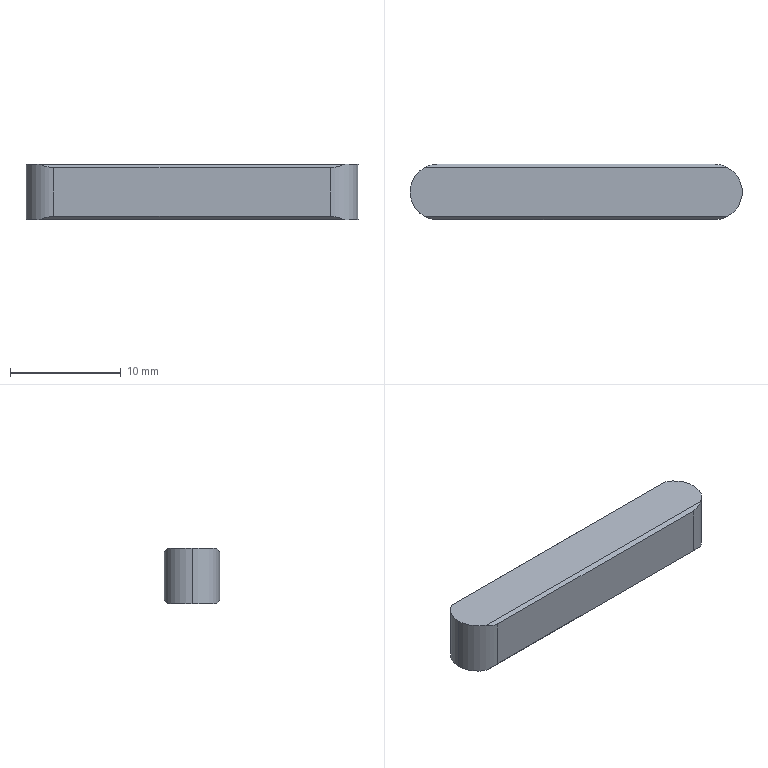Part | STEP file | 0245_004_KESS5-30 | 1 solid | 11 faces | box 30 x 5 x 5 mm | volume 718.443 mm3 | plane 8 | cylinder 3 | commonest cylinder face diameters 5 x3
STEP:
#1=CARTESIAN_POINT('',(0.,0.,0.));
#2=DIRECTION('',(0.,0.,1.));
#3=DIRECTION('',(1.,0.,0.));
#4=AXIS2_PLACEMENT_3D('',#1,#2,#3);
#5=CARTESIAN_POINT('',(0.,2.5,5.));
#6=VERTEX_POINT('',#5);
#7=CARTESIAN_POINT('',(1.313,0.3,5.));
#8=VERTEX_POINT('',#7);
#9=CARTESIAN_POINT('',(2.5,2.5,5.));
#10=DIRECTION('',(0.,0.,1.));
#11=DIRECTION('',(-1.,0.,0.));
#12=AXIS2_PLACEMENT_3D('',#9,#10,#11);
#13=CIRCLE('',#12,2.5);
#14=CARTESIAN_POINT('',(2.5,2.5,0.));
#15=DIRECTION('',(0.,0.,-1.));
#16=DIRECTION('',(-1.,0.,0.));
#17=AXIS2_PLACEMENT_3D('',#14,#15,#16);
#18=CYLINDRICAL_SURFACE('',#17,2.5);
#19=CARTESIAN_POINT('',(6.283,-5.));
#20=DIRECTION('',(-1.,0.));
#21=VECTOR('',#20,1.);
#22=LINE('',#19,#21);
#23=(GEOMETRIC_REPRESENTATION_CONTEXT(2)PARAMETRIC_REPRESENTATION_CONTEXT()REPRESENTATION_CONTEXT('',''));
#24=DEFINITIONAL_REPRESENTATION('',(#22),#23);
#25=PCURVE('',#18,#24);
#26=CARTESIAN_POINT('',(0.,0.,5.));
#27=DIRECTION('',(0.,0.,1.));
#28=DIRECTION('',(1.,0.,0.));
#29=AXIS2_PLACEMENT_3D('',#26,#27,#28);
#30=PLANE('',#29);
#31=CARTESIAN_POINT('',(2.5,2.5));
#32=DIRECTION('',(-1.,0.));
#33=AXIS2_PLACEMENT_2D('',#31,#32);
#34=CIRCLE('',#33,2.5);
#35=(GEOMETRIC_REPRESENTATION_CONTEXT(2)PARAMETRIC_REPRESENTATION_CONTEXT()REPRESENTATION_CONTEXT('',''));
#36=DEFINITIONAL_REPRESENTATION('',(#34),#35);
#37=PCURVE('',#30,#36);
#38=SURFACE_CURVE('',#13,(#25,#37),.PCURVE_S1.);
#39=EDGE_CURVE('',#6,#8,#38,.T.);
#40=ORIENTED_EDGE('',*,*,#39,.F.);
#41=CARTESIAN_POINT('',(0.,2.5,0.));
#42=VERTEX_POINT('',#41);
#43=CARTESIAN_POINT('',(0.,2.5,0.));
#44=DIRECTION('',(0.,0.,-1.));
#45=VECTOR('',#44,1.);
#46=LINE('',#43,#45);
#47=CARTESIAN_POINT('',(6.283,0.));
#48=DIRECTION('',(0.,1.));
#49=VECTOR('',#48,1.);
#50=LINE('',#47,#49);
#51=(GEOMETRIC_REPRESENTATION_CONTEXT(2)PARAMETRIC_REPRESENTATION_CONTEXT()REPRESENTATION_CONTEXT('',''));
#52=DEFINITIONAL_REPRESENTATION('',(#50),#51);
#53=PCURVE('',#18,#52);
#54=CARTESIAN_POINT('',(2.5,2.5,0.));
#55=DIRECTION('',(0.,0.,-1.));
#56=DIRECTION('',(-1.,0.,0.));
#57=AXIS2_PLACEMENT_3D('',#54,#55,#56);
#58=CYLINDRICAL_SURFACE('',#57,2.5);
#59=CARTESIAN_POINT('',(0.,0.));
#60=DIRECTION('',(0.,1.));
#61=VECTOR('',#60,1.);
#62=LINE('',#59,#61);
#63=(GEOMETRIC_REPRESENTATION_CONTEXT(2)PARAMETRIC_REPRESENTATION_CONTEXT()REPRESENTATION_CONTEXT('',''));
#64=DEFINITIONAL_REPRESENTATION('',(#62),#63);
#65=PCURVE('',#58,#64);
#66=SURFACE_CURVE('',#46,(#53,#65),.PCURVE_S1.);
#67=EDGE_CURVE('',#6,#42,#66,.T.);
#68=ORIENTED_EDGE('',*,*,#67,.T.);
#69=CARTESIAN_POINT('',(1.313,0.3,0.));
#70=VERTEX_POINT('',#69);
#71=CARTESIAN_POINT('',(2.5,2.5,0.));
#72=DIRECTION('',(0.,0.,1.));
#73=DIRECTION('',(-1.,0.,0.));
#74=AXIS2_PLACEMENT_3D('',#71,#72,#73);
#75=CIRCLE('',#74,2.5);
#76=CARTESIAN_POINT('',(6.283,0.));
#77=DIRECTION('',(-1.,0.));
#78=VECTOR('',#77,1.);
#79=LINE('',#76,#78);
#80=(GEOMETRIC_REPRESENTATION_CONTEXT(2)PARAMETRIC_REPRESENTATION_CONTEXT()REPRESENTATION_CONTEXT('',''));
#81=DEFINITIONAL_REPRESENTATION('',(#79),#80);
#82=PCURVE('',#18,#81);
#83=CARTESIAN_POINT('',(0.,0.,0.));
#84=DIRECTION('',(0.,0.,1.));
#85=DIRECTION('',(1.,0.,0.));
#86=AXIS2_PLACEMENT_3D('',#83,#84,#85);
#87=PLANE('',#86);
#88=CARTESIAN_POINT('',(2.5,2.5));
#89=DIRECTION('',(-1.,0.));
#90=AXIS2_PLACEMENT_2D('',#88,#89);
#91=CIRCLE('',#90,2.5);
#92=(GEOMETRIC_REPRESENTATION_CONTEXT(2)PARAMETRIC_REPRESENTATION_CONTEXT()REPRESENTATION_CONTEXT('',''));
#93=DEFINITIONAL_REPRESENTATION('',(#91),#92);
#94=PCURVE('',#87,#93);
#95=SURFACE_CURVE('',#75,(#82,#94),.PCURVE_S1.);
#96=EDGE_CURVE('',#42,#70,#95,.T.);
#97=ORIENTED_EDGE('',*,*,#96,.T.);
#98=CARTESIAN_POINT('',(2.5,0.,0.3));
#99=VERTEX_POINT('',#98);
#100=CARTESIAN_POINT('',(1.313,0.3,0.));
#101=CARTESIAN_POINT('',(1.679,0.1021,0.1979));
#102=CARTESIAN_POINT('',(2.083,0.,0.3));
#103=CARTESIAN_POINT('',(2.5,0.,0.3));
#104=(BOUNDED_CURVE()B_SPLINE_CURVE(3,(#100,#101,#102,#103),.UNSPECIFIED.,.F.,.F.)B_SPLINE_CURVE_WITH_KNOTS((4,4),(2.647,3.142),.PIECEWISE_BEZIER_KNOTS.)CURVE()GEOMETRIC_REPRESENTATION_ITEM()RATIONAL_B_SPLINE_CURVE((1.,0.9797,0.9797,1.))REPRESENTATION_ITEM(''));
#105=CARTESIAN_POINT('',(5.207,0.));
#106=CARTESIAN_POINT('',(5.2,-0.008814));
#107=CARTESIAN_POINT('',(5.185,-0.0261));
#108=CARTESIAN_POINT('',(5.163,-0.05099));
#109=CARTESIAN_POINT('',(5.14,-0.07481));
#110=CARTESIAN_POINT('',(5.118,-0.09752));
#111=CARTESIAN_POINT('',(5.095,-0.1191));
#112=CARTESIAN_POINT('',(5.073,-0.1396));
#113=CARTESIAN_POINT('',(5.05,-0.1589));
#114=CARTESIAN_POINT('',(5.028,-0.177));
#115=CARTESIAN_POINT('',(5.005,-0.1939));
#116=CARTESIAN_POINT('',(4.982,-0.2096));
#117=CARTESIAN_POINT('',(4.96,-0.224));
#118=CARTESIAN_POINT('',(4.937,-0.2373));
#119=CARTESIAN_POINT('',(4.915,-0.2493));
#120=CARTESIAN_POINT('',(4.892,-0.26));
#121=CARTESIAN_POINT('',(4.869,-0.2694));
#122=CARTESIAN_POINT('',(4.847,-0.2776));
#123=CARTESIAN_POINT('',(4.824,-0.2845));
#124=CARTESIAN_POINT('',(4.802,-0.2902));
#125=CARTESIAN_POINT('',(4.779,-0.2946));
#126=CARTESIAN_POINT('',(4.757,-0.2977));
#127=CARTESIAN_POINT('',(4.735,-0.2996));
#128=CARTESIAN_POINT('',(4.72,-0.3));
#129=CARTESIAN_POINT('',(4.712,-0.3));
#130=B_SPLINE_CURVE_WITH_KNOTS('',3,(#105,#106,#107,#108,#109,#110,#111,#112,#113,#114,#115,#116,#117,#118,#119,#120,#121,#122,#123,#124,#125,#126,#127,#128,#129),.UNSPECIFIED.,.F.,.F.,(4,1,1,1,1,1,1,1,1,1,1,1,1,1,1,1,1,1,1,1,1,1,4),(2.647,2.669,2.692,2.714,2.737,2.759,2.782,2.804,2.827,2.849,2.872,2.894,2.917,2.939,2.962,2.984,3.007,3.029,3.052,3.074,3.097,3.119,3.142),.QUASI_UNIFORM_KNOTS.);
#131=(GEOMETRIC_REPRESENTATION_CONTEXT(2)PARAMETRIC_REPRESENTATION_CONTEXT()REPRESENTATION_CONTEXT('',''));
#132=DEFINITIONAL_REPRESENTATION('',(#130),#131);
#133=PCURVE('',#18,#132);
#134=CARTESIAN_POINT('',(0.,0.,0.3));
#135=DIRECTION('',(0.,0.7071,0.7071));
#136=DIRECTION('',(0.,-0.7071,0.7071));
#137=AXIS2_PLACEMENT_3D('',#134,#135,#136);
#138=PLANE('',#137);
#139=CARTESIAN_POINT('',(-0.4243,1.313));
#140=CARTESIAN_POINT('',(-0.1444,1.679));
#141=CARTESIAN_POINT('',(0.,2.083));
#142=CARTESIAN_POINT('',(0.,2.5));
#143=(BOUNDED_CURVE()B_SPLINE_CURVE(3,(#139,#140,#141,#142),.UNSPECIFIED.,.F.,.F.)B_SPLINE_CURVE_WITH_KNOTS((4,4),(2.647,3.142),.PIECEWISE_BEZIER_KNOTS.)CURVE()GEOMETRIC_REPRESENTATION_ITEM()RATIONAL_B_SPLINE_CURVE((1.,0.9797,0.9797,1.))REPRESENTATION_ITEM(''));
#144=(GEOMETRIC_REPRESENTATION_CONTEXT(2)PARAMETRIC_REPRESENTATION_CONTEXT()REPRESENTATION_CONTEXT('',''));
#145=DEFINITIONAL_REPRESENTATION('',(#143),#144);
#146=PCURVE('',#138,#145);
#147=SURFACE_CURVE('',#104,(#133,#146),.PCURVE_S1.);
#148=EDGE_CURVE('',#70,#99,#147,.T.);
#149=ORIENTED_EDGE('',*,*,#148,.T.);
#150=CARTESIAN_POINT('',(2.5,0.,4.7));
#151=VERTEX_POINT('',#150);
#152=CARTESIAN_POINT('',(2.5,0.,0.));
#153=DIRECTION('',(0.,0.,1.));
#154=VECTOR('',#153,1.);
#155=LINE('',#152,#154);
#156=CARTESIAN_POINT('',(4.712,0.));
#157=DIRECTION('',(0.,-1.));
#158=VECTOR('',#157,1.);
#159=LINE('',#156,#158);
#160=(GEOMETRIC_REPRESENTATION_CONTEXT(2)PARAMETRIC_REPRESENTATION_CONTEXT()REPRESENTATION_CONTEXT('',''));
#161=DEFINITIONAL_REPRESENTATION('',(#159),#160);
#162=PCURVE('',#18,#161);
#163=CARTESIAN_POINT('',(27.5,0.,0.));
#164=DIRECTION('',(0.,-1.,0.));
#165=DIRECTION('',(0.,0.,-1.));
#166=AXIS2_PLACEMENT_3D('',#163,#164,#165);
#167=PLANE('',#166);
#168=CARTESIAN_POINT('',(0.,-25.));
#169=DIRECTION('',(-1.,0.));
#170=VECTOR('',#169,1.);
#171=LINE('',#168,#170);
#172=(GEOMETRIC_REPRESENTATION_CONTEXT(2)PARAMETRIC_REPRESENTATION_CONTEXT()REPRESENTATION_CONTEXT('',''));
#173=DEFINITIONAL_REPRESENTATION('',(#171),#172);
#174=PCURVE('',#167,#173);
#175=SURFACE_CURVE('',#155,(#162,#174),.PCURVE_S1.);
#176=EDGE_CURVE('',#99,#151,#175,.T.);
#177=ORIENTED_EDGE('',*,*,#176,.T.);
#178=CARTESIAN_POINT('',(2.5,0.,4.7));
#179=CARTESIAN_POINT('',(2.083,0.,4.7));
#180=CARTESIAN_POINT('',(1.679,0.1021,4.802));
#181=CARTESIAN_POINT('',(1.313,0.3,5.));
#182=(BOUNDED_CURVE()B_SPLINE_CURVE(3,(#178,#179,#180,#181),.UNSPECIFIED.,.F.,.F.)B_SPLINE_CURVE_WITH_KNOTS((4,4),(0.,0.4949),.PIECEWISE_BEZIER_KNOTS.)CURVE()GEOMETRIC_REPRESENTATION_ITEM()RATIONAL_B_SPLINE_CURVE((1.,0.9797,0.9797,1.))REPRESENTATION_ITEM(''));
#183=CARTESIAN_POINT('',(4.712,-4.7));
#184=CARTESIAN_POINT('',(4.72,-4.7));
#185=CARTESIAN_POINT('',(4.735,-4.7));
#186=CARTESIAN_POINT('',(4.757,-4.702));
#187=CARTESIAN_POINT('',(4.779,-4.705));
#188=CARTESIAN_POINT('',(4.802,-4.71));
#189=CARTESIAN_POINT('',(4.824,-4.715));
#190=CARTESIAN_POINT('',(4.847,-4.722));
#191=CARTESIAN_POINT('',(4.869,-4.731));
#192=CARTESIAN_POINT('',(4.892,-4.74));
#193=CARTESIAN_POINT('',(4.915,-4.751));
#194=CARTESIAN_POINT('',(4.937,-4.763));
#195=CARTESIAN_POINT('',(4.96,-4.776));
#196=CARTESIAN_POINT('',(4.982,-4.79));
#197=CARTESIAN_POINT('',(5.005,-4.806));
#198=CARTESIAN_POINT('',(5.028,-4.823));
#199=CARTESIAN_POINT('',(5.05,-4.841));
#200=CARTESIAN_POINT('',(5.073,-4.86));
#201=CARTESIAN_POINT('',(5.095,-4.881));
#202=CARTESIAN_POINT('',(5.118,-4.902));
#203=CARTESIAN_POINT('',(5.14,-4.925));
#204=CARTESIAN_POINT('',(5.163,-4.949));
#205=CARTESIAN_POINT('',(5.185,-4.974));
#206=CARTESIAN_POINT('',(5.2,-4.991));
#207=CARTESIAN_POINT('',(5.207,-5.));
#208=B_SPLINE_CURVE_WITH_KNOTS('',3,(#183,#184,#185,#186,#187,#188,#189,#190,#191,#192,#193,#194,#195,#196,#197,#198,#199,#200,#201,#202,#203,#204,#205,#206,#207),.UNSPECIFIED.,.F.,.F.,(4,1,1,1,1,1,1,1,1,1,1,1,1,1,1,1,1,1,1,1,1,1,4),(0.,0.0225,0.04499,0.06749,0.08999,0.1125,0.135,0.1575,0.18,0.2025,0.225,0.2475,0.27,0.2925,0.315,0.3375,0.36,0.3824,0.4049,0.4274,0.4499,0.4724,0.4949),.QUASI_UNIFORM_KNOTS.);
#209=(GEOMETRIC_REPRESENTATION_CONTEXT(2)PARAMETRIC_REPRESENTATION_CONTEXT()REPRESENTATION_CONTEXT('',''));
#210=DEFINITIONAL_REPRESENTATION('',(#208),#209);
#211=PCURVE('',#18,#210);
#212=CARTESIAN_POINT('',(0.,0.3,5.));
#213=DIRECTION('',(0.,0.7071,-0.7071));
#214=DIRECTION('',(0.,0.7071,0.7071));
#215=AXIS2_PLACEMENT_3D('',#212,#213,#214);
#216=PLANE('',#215);
#217=CARTESIAN_POINT('',(-0.4243,2.5));
#218=CARTESIAN_POINT('',(-0.4243,2.083));
#219=CARTESIAN_POINT('',(-0.2799,1.679));
#220=CARTESIAN_POINT('',(0.,1.313));
#221=(BOUNDED_CURVE()B_SPLINE_CURVE(3,(#217,#218,#219,#220),.UNSPECIFIED.,.F.,.F.)B_SPLINE_CURVE_WITH_KNOTS((4,4),(0.,0.4949),.PIECEWISE_BEZIER_KNOTS.)CURVE()GEOMETRIC_REPRESENTATION_ITEM()RATIONAL_B_SPLINE_CURVE((1.,0.9797,0.9797,1.))REPRESENTATION_ITEM(''));
#222=(GEOMETRIC_REPRESENTATION_CONTEXT(2)PARAMETRIC_REPRESENTATION_CONTEXT()REPRESENTATION_CONTEXT('',''));
#223=DEFINITIONAL_REPRESENTATION('',(#221),#222);
#224=PCURVE('',#216,#223);
#225=SURFACE_CURVE('',#182,(#211,#224),.PCURVE_S1.);
#226=EDGE_CURVE('',#151,#8,#225,.T.);
#227=ORIENTED_EDGE('',*,*,#226,.T.);
#228=EDGE_LOOP('',(#40,#68,#97,#149,#177,#227));
#229=FACE_BOUND('',#228,.T.);
#230=ADVANCED_FACE('',(#229),#18,.T.);
#231=CARTESIAN_POINT('',(28.687,4.7,5.));
#232=VERTEX_POINT('',#231);
#233=CARTESIAN_POINT('',(1.313,4.7,5.));
#234=VERTEX_POINT('',#233);
#235=CARTESIAN_POINT('',(0.,4.7,5.));
#236=DIRECTION('',(-1.,0.,0.));
#237=VECTOR('',#236,1.);
#238=LINE('',#235,#237);
#239=CARTESIAN_POINT('',(0.,4.7));
#240=DIRECTION('',(-1.,0.));
#241=VECTOR('',#240,1.);
#242=LINE('',#239,#241);
#243=(GEOMETRIC_REPRESENTATION_CONTEXT(2)PARAMETRIC_REPRESENTATION_CONTEXT()REPRESENTATION_CONTEXT('',''));
#244=DEFINITIONAL_REPRESENTATION('',(#242),#243);
#245=PCURVE('',#30,#244);
#246=CARTESIAN_POINT('',(0.,5.,4.7));
#247=DIRECTION('',(0.,-0.7071,-0.7071));
#248=DIRECTION('',(0.,0.7071,-0.7071));
#249=AXIS2_PLACEMENT_3D('',#246,#247,#248);
#250=PLANE('',#249);
#251=CARTESIAN_POINT('',(-0.4243,0.));
#252=DIRECTION('',(0.,-1.));
#253=VECTOR('',#252,1.);
#254=LINE('',#251,#253);
#255=(GEOMETRIC_REPRESENTATION_CONTEXT(2)PARAMETRIC_REPRESENTATION_CONTEXT()REPRESENTATION_CONTEXT('',''));
#256=DEFINITIONAL_REPRESENTATION('',(#254),#255);
#257=PCURVE('',#250,#256);
#258=SURFACE_CURVE('',#238,(#245,#257),.PCURVE_S1.);
#259=EDGE_CURVE('',#232,#234,#258,.T.);
#260=ORIENTED_EDGE('',*,*,#259,.T.);
#261=CARTESIAN_POINT('',(2.5,2.5,5.));
#262=DIRECTION('',(0.,0.,1.));
#263=DIRECTION('',(-1.,0.,0.));
#264=AXIS2_PLACEMENT_3D('',#261,#262,#263);
#265=CIRCLE('',#264,2.5);
#266=CARTESIAN_POINT('',(2.5,2.5));
#267=DIRECTION('',(-1.,0.));
#268=AXIS2_PLACEMENT_2D('',#266,#267);
#269=CIRCLE('',#268,2.5);
#270=(GEOMETRIC_REPRESENTATION_CONTEXT(2)PARAMETRIC_REPRESENTATION_CONTEXT()REPRESENTATION_CONTEXT('',''));
#271=DEFINITIONAL_REPRESENTATION('',(#269),#270);
#272=PCURVE('',#30,#271);
#273=CARTESIAN_POINT('',(6.283,-5.));
#274=DIRECTION('',(-1.,0.));
#275=VECTOR('',#274,1.);
#276=LINE('',#273,#275);
#277=(GEOMETRIC_REPRESENTATION_CONTEXT(2)PARAMETRIC_REPRESENTATION_CONTEXT()REPRESENTATION_CONTEXT('',''));
#278=DEFINITIONAL_REPRESENTATION('',(#276),#277);
#279=PCURVE('',#58,#278);
#280=SURFACE_CURVE('',#265,(#272,#279),.PCURVE_S1.);
#281=EDGE_CURVE('',#234,#6,#280,.T.);
#282=ORIENTED_EDGE('',*,*,#281,.T.);
#283=ORIENTED_EDGE('',*,*,#39,.T.);
#284=CARTESIAN_POINT('',(28.687,0.3,5.));
#285=VERTEX_POINT('',#284);
#286=CARTESIAN_POINT('',(0.,0.3,5.));
#287=DIRECTION('',(1.,0.,0.));
#288=VECTOR('',#287,1.);
#289=LINE('',#286,#288);
#290=CARTESIAN_POINT('',(0.,0.3));
#291=DIRECTION('',(1.,0.));
#292=VECTOR('',#291,1.);
#293=LINE('',#290,#292);
#294=(GEOMETRIC_REPRESENTATION_CONTEXT(2)PARAMETRIC_REPRESENTATION_CONTEXT()REPRESENTATION_CONTEXT('',''));
#295=DEFINITIONAL_REPRESENTATION('',(#293),#294);
#296=PCURVE('',#30,#295);
#297=CARTESIAN_POINT('',(0.,0.));
#298=DIRECTION('',(0.,1.));
#299=VECTOR('',#298,1.);
#300=LINE('',#297,#299);
#301=(GEOMETRIC_REPRESENTATION_CONTEXT(2)PARAMETRIC_REPRESENTATION_CONTEXT()REPRESENTATION_CONTEXT('',''));
#302=DEFINITIONAL_REPRESENTATION('',(#300),#301);
#303=PCURVE('',#216,#302);
#304=SURFACE_CURVE('',#289,(#296,#303),.PCURVE_S1.);
#305=EDGE_CURVE('',#8,#285,#304,.T.);
#306=ORIENTED_EDGE('',*,*,#305,.T.);
#307=CARTESIAN_POINT('',(27.5,2.5,5.));
#308=DIRECTION('',(0.,0.,1.));
#309=DIRECTION('',(-1.,0.,0.));
#310=AXIS2_PLACEMENT_3D('',#307,#308,#309);
#311=CIRCLE('',#310,2.5);
#312=CARTESIAN_POINT('',(27.5,2.5));
#313=DIRECTION('',(-1.,0.));
#314=AXIS2_PLACEMENT_2D('',#312,#313);
#315=CIRCLE('',#314,2.5);
#316=(GEOMETRIC_REPRESENTATION_CONTEXT(2)PARAMETRIC_REPRESENTATION_CONTEXT()REPRESENTATION_CONTEXT('',''));
#317=DEFINITIONAL_REPRESENTATION('',(#315),#316);
#318=PCURVE('',#30,#317);
#319=CARTESIAN_POINT('',(27.5,2.5,0.));
#320=DIRECTION('',(0.,0.,-1.));
#321=DIRECTION('',(-1.,0.,0.));
#322=AXIS2_PLACEMENT_3D('',#319,#320,#321);
#323=CYLINDRICAL_SURFACE('',#322,2.5);
#324=CARTESIAN_POINT('',(6.283,-5.));
#325=DIRECTION('',(-1.,0.));
#326=VECTOR('',#325,1.);
#327=LINE('',#324,#326);
#328=(GEOMETRIC_REPRESENTATION_CONTEXT(2)PARAMETRIC_REPRESENTATION_CONTEXT()REPRESENTATION_CONTEXT('',''));
#329=DEFINITIONAL_REPRESENTATION('',(#327),#328);
#330=PCURVE('',#323,#329);
#331=SURFACE_CURVE('',#311,(#318,#330),.PCURVE_S1.);
#332=EDGE_CURVE('',#285,#232,#331,.T.);
#333=ORIENTED_EDGE('',*,*,#332,.T.);
#334=EDGE_LOOP('',(#260,#282,#283,#306,#333));
#335=FACE_BOUND('',#334,.T.);
#336=ADVANCED_FACE('',(#335),#30,.T.);
#337=ORIENTED_EDGE('',*,*,#67,.F.);
#338=ORIENTED_EDGE('',*,*,#281,.F.);
#339=CARTESIAN_POINT('',(2.5,5.,4.7));
#340=VERTEX_POINT('',#339);
#341=CARTESIAN_POINT('',(1.313,4.7,5.));
#342=CARTESIAN_POINT('',(1.679,4.898,4.802));
#343=CARTESIAN_POINT('',(2.083,5.,4.7));
#344=CARTESIAN_POINT('',(2.5,5.,4.7));
#345=(BOUNDED_CURVE()B_SPLINE_CURVE(3,(#341,#342,#343,#344),.UNSPECIFIED.,.F.,.F.)B_SPLINE_CURVE_WITH_KNOTS((4,4),(5.788,6.283),.PIECEWISE_BEZIER_KNOTS.)CURVE()GEOMETRIC_REPRESENTATION_ITEM()RATIONAL_B_SPLINE_CURVE((1.,0.9797,0.9797,1.))REPRESENTATION_ITEM(''));
#346=CARTESIAN_POINT('',(1.076,-5.));
#347=CARTESIAN_POINT('',(1.083,-4.991));
#348=CARTESIAN_POINT('',(1.098,-4.974));
#349=CARTESIAN_POINT('',(1.121,-4.949));
#350=CARTESIAN_POINT('',(1.143,-4.925));
#351=CARTESIAN_POINT('',(1.165,-4.902));
#352=CARTESIAN_POINT('',(1.188,-4.881));
#353=CARTESIAN_POINT('',(1.21,-4.86));
#354=CARTESIAN_POINT('',(1.233,-4.841));
#355=CARTESIAN_POINT('',(1.256,-4.823));
#356=CARTESIAN_POINT('',(1.278,-4.806));
#357=CARTESIAN_POINT('',(1.301,-4.79));
#358=CARTESIAN_POINT('',(1.323,-4.776));
#359=CARTESIAN_POINT('',(1.346,-4.763));
#360=CARTESIAN_POINT('',(1.369,-4.751));
#361=CARTESIAN_POINT('',(1.391,-4.74));
#362=CARTESIAN_POINT('',(1.414,-4.731));
#363=CARTESIAN_POINT('',(1.436,-4.722));
#364=CARTESIAN_POINT('',(1.459,-4.715));
#365=CARTESIAN_POINT('',(1.481,-4.71));
#366=CARTESIAN_POINT('',(1.504,-4.705));
#367=CARTESIAN_POINT('',(1.526,-4.702));
#368=CARTESIAN_POINT('',(1.549,-4.7));
#369=CARTESIAN_POINT('',(1.563,-4.7));
#370=CARTESIAN_POINT('',(1.571,-4.7));
#371=B_SPLINE_CURVE_WITH_KNOTS('',3,(#346,#347,#348,#349,#350,#351,#352,#353,#354,#355,#356,#357,#358,#359,#360,#361,#362,#363,#364,#365,#366,#367,#368,#369,#370),.UNSPECIFIED.,.F.,.F.,(4,1,1,1,1,1,1,1,1,1,1,1,1,1,1,1,1,1,1,1,1,1,4),(5.788,5.811,5.833,5.856,5.878,5.901,5.923,5.946,5.968,5.991,6.013,6.036,6.058,6.081,6.103,6.126,6.148,6.171,6.193,6.216,6.238,6.261,6.283),.QUASI_UNIFORM_KNOTS.);
#372=(GEOMETRIC_REPRESENTATION_CONTEXT(2)PARAMETRIC_REPRESENTATION_CONTEXT()REPRESENTATION_CONTEXT('',''));
#373=DEFINITIONAL_REPRESENTATION('',(#371),#372);
#374=PCURVE('',#58,#373);
#375=CARTESIAN_POINT('',(-0.4243,1.313));
#376=CARTESIAN_POINT('',(-0.1444,1.679));
#377=CARTESIAN_POINT('',(0.,2.083));
#378=CARTESIAN_POINT('',(0.,2.5));
#379=(BOUNDED_CURVE()B_SPLINE_CURVE(3,(#375,#376,#377,#378),.UNSPECIFIED.,.F.,.F.)B_SPLINE_CURVE_WITH_KNOTS((4,4),(5.788,6.283),.PIECEWISE_BEZIER_KNOTS.)CURVE()GEOMETRIC_REPRESENTATION_ITEM()RATIONAL_B_SPLINE_CURVE((1.,0.9797,0.9797,1.))REPRESENTATION_ITEM(''));
#380=(GEOMETRIC_REPRESENTATION_CONTEXT(2)PARAMETRIC_REPRESENTATION_CONTEXT()REPRESENTATION_CONTEXT('',''));
#381=DEFINITIONAL_REPRESENTATION('',(#379),#380);
#382=PCURVE('',#250,#381);
#383=SURFACE_CURVE('',#345,(#374,#382),.PCURVE_S1.);
#384=EDGE_CURVE('',#234,#340,#383,.T.);
#385=ORIENTED_EDGE('',*,*,#384,.T.);
#386=CARTESIAN_POINT('',(2.5,5.,0.3));
#387=VERTEX_POINT('',#386);
#388=CARTESIAN_POINT('',(2.5,5.,0.));
#389=DIRECTION('',(0.,0.,-1.));
#390=VECTOR('',#389,1.);
#391=LINE('',#388,#390);
#392=CARTESIAN_POINT('',(1.571,0.));
#393=DIRECTION('',(0.,1.));
#394=VECTOR('',#393,1.);
#395=LINE('',#392,#394);
#396=(GEOMETRIC_REPRESENTATION_CONTEXT(2)PARAMETRIC_REPRESENTATION_CONTEXT()REPRESENTATION_CONTEXT('',''));
#397=DEFINITIONAL_REPRESENTATION('',(#395),#396);
#398=PCURVE('',#58,#397);
#399=CARTESIAN_POINT('',(2.5,5.,0.));
#400=DIRECTION('',(0.,1.,0.));
#401=DIRECTION('',(0.,0.,1.));
#402=AXIS2_PLACEMENT_3D('',#399,#400,#401);
#403=PLANE('',#402);
#404=CARTESIAN_POINT('',(0.,0.));
#405=DIRECTION('',(-1.,0.));
#406=VECTOR('',#405,1.);
#407=LINE('',#404,#406);
#408=(GEOMETRIC_REPRESENTATION_CONTEXT(2)PARAMETRIC_REPRESENTATION_CONTEXT()REPRESENTATION_CONTEXT('',''));
#409=DEFINITIONAL_REPRESENTATION('',(#407),#408);
#410=PCURVE('',#403,#409);
#411=SURFACE_CURVE('',#391,(#398,#410),.PCURVE_S1.);
#412=EDGE_CURVE('',#340,#387,#411,.T.);
#413=ORIENTED_EDGE('',*,*,#412,.T.);
#414=CARTESIAN_POINT('',(1.313,4.7,0.));
#415=VERTEX_POINT('',#414);
#416=CARTESIAN_POINT('',(2.5,5.,0.3));
#417=CARTESIAN_POINT('',(2.083,5.,0.3));
#418=CARTESIAN_POINT('',(1.679,4.898,0.1979));
#419=CARTESIAN_POINT('',(1.313,4.7,0.));
#420=(BOUNDED_CURVE()B_SPLINE_CURVE(3,(#416,#417,#418,#419),.UNSPECIFIED.,.F.,.F.)B_SPLINE_CURVE_WITH_KNOTS((4,4),(3.142,3.637),.PIECEWISE_BEZIER_KNOTS.)CURVE()GEOMETRIC_REPRESENTATION_ITEM()RATIONAL_B_SPLINE_CURVE((1.,0.9797,0.9797,1.))REPRESENTATION_ITEM(''));
#421=CARTESIAN_POINT('',(1.571,-0.3));
#422=CARTESIAN_POINT('',(1.563,-0.3));
#423=CARTESIAN_POINT('',(1.549,-0.2996));
#424=CARTESIAN_POINT('',(1.526,-0.2977));
#425=CARTESIAN_POINT('',(1.504,-0.2946));
#426=CARTESIAN_POINT('',(1.481,-0.2902));
#427=CARTESIAN_POINT('',(1.459,-0.2845));
#428=CARTESIAN_POINT('',(1.436,-0.2776));
#429=CARTESIAN_POINT('',(1.414,-0.2694));
#430=CARTESIAN_POINT('',(1.391,-0.26));
#431=CARTESIAN_POINT('',(1.369,-0.2493));
#432=CARTESIAN_POINT('',(1.346,-0.2373));
#433=CARTESIAN_POINT('',(1.323,-0.224));
#434=CARTESIAN_POINT('',(1.301,-0.2096));
#435=CARTESIAN_POINT('',(1.278,-0.1939));
#436=CARTESIAN_POINT('',(1.256,-0.177));
#437=CARTESIAN_POINT('',(1.233,-0.1589));
#438=CARTESIAN_POINT('',(1.21,-0.1396));
#439=CARTESIAN_POINT('',(1.188,-0.1191));
#440=CARTESIAN_POINT('',(1.165,-0.09752));
#441=CARTESIAN_POINT('',(1.143,-0.07481));
#442=CARTESIAN_POINT('',(1.121,-0.05099));
#443=CARTESIAN_POINT('',(1.098,-0.0261));
#444=CARTESIAN_POINT('',(1.083,-0.008814));
#445=CARTESIAN_POINT('',(1.076,0.));
#446=B_SPLINE_CURVE_WITH_KNOTS('',3,(#421,#422,#423,#424,#425,#426,#427,#428,#429,#430,#431,#432,#433,#434,#435,#436,#437,#438,#439,#440,#441,#442,#443,#444,#445),.UNSPECIFIED.,.F.,.F.,(4,1,1,1,1,1,1,1,1,1,1,1,1,1,1,1,1,1,1,1,1,1,4),(3.142,3.164,3.187,3.209,3.232,3.254,3.277,3.299,3.322,3.344,3.367,3.389,3.412,3.434,3.457,3.479,3.502,3.524,3.547,3.569,3.592,3.614,3.637),.QUASI_UNIFORM_KNOTS.);
#447=(GEOMETRIC_REPRESENTATION_CONTEXT(2)PARAMETRIC_REPRESENTATION_CONTEXT()REPRESENTATION_CONTEXT('',''));
#448=DEFINITIONAL_REPRESENTATION('',(#446),#447);
#449=PCURVE('',#58,#448);
#450=CARTESIAN_POINT('',(0.,4.7,0.));
#451=DIRECTION('',(0.,-0.7071,0.7071));
#452=DIRECTION('',(0.,-0.7071,-0.7071));
#453=AXIS2_PLACEMENT_3D('',#450,#451,#452);
#454=PLANE('',#453);
#455=CARTESIAN_POINT('',(-0.4243,2.5));
#456=CARTESIAN_POINT('',(-0.4243,2.083));
#457=CARTESIAN_POINT('',(-0.2799,1.679));
#458=CARTESIAN_POINT('',(0.,1.313));
#459=(BOUNDED_CURVE()B_SPLINE_CURVE(3,(#455,#456,#457,#458),.UNSPECIFIED.,.F.,.F.)B_SPLINE_CURVE_WITH_KNOTS((4,4),(3.142,3.637),.PIECEWISE_BEZIER_KNOTS.)CURVE()GEOMETRIC_REPRESENTATION_ITEM()RATIONAL_B_SPLINE_CURVE((1.,0.9797,0.9797,1.))REPRESENTATION_ITEM(''));
#460=(GEOMETRIC_REPRESENTATION_CONTEXT(2)PARAMETRIC_REPRESENTATION_CONTEXT()REPRESENTATION_CONTEXT('',''));
#461=DEFINITIONAL_REPRESENTATION('',(#459),#460);
#462=PCURVE('',#454,#461);
#463=SURFACE_CURVE('',#420,(#449,#462),.PCURVE_S1.);
#464=EDGE_CURVE('',#387,#415,#463,.T.);
#465=ORIENTED_EDGE('',*,*,#464,.T.);
#466=CARTESIAN_POINT('',(2.5,2.5,0.));
#467=DIRECTION('',(0.,0.,1.));
#468=DIRECTION('',(-1.,0.,0.));
#469=AXIS2_PLACEMENT_3D('',#466,#467,#468);
#470=CIRCLE('',#469,2.5);
#471=CARTESIAN_POINT('',(6.283,0.));
#472=DIRECTION('',(-1.,0.));
#473=VECTOR('',#472,1.);
#474=LINE('',#471,#473);
#475=(GEOMETRIC_REPRESENTATION_CONTEXT(2)PARAMETRIC_REPRESENTATION_CONTEXT()REPRESENTATION_CONTEXT('',''));
#476=DEFINITIONAL_REPRESENTATION('',(#474),#475);
#477=PCURVE('',#58,#476);
#478=CARTESIAN_POINT('',(2.5,2.5));
#479=DIRECTION('',(-1.,0.));
#480=AXIS2_PLACEMENT_2D('',#478,#479);
#481=CIRCLE('',#480,2.5);
#482=(GEOMETRIC_REPRESENTATION_CONTEXT(2)PARAMETRIC_REPRESENTATION_CONTEXT()REPRESENTATION_CONTEXT('',''));
#483=DEFINITIONAL_REPRESENTATION('',(#481),#482);
#484=PCURVE('',#87,#483);
#485=SURFACE_CURVE('',#470,(#477,#484),.PCURVE_S1.);
#486=EDGE_CURVE('',#415,#42,#485,.T.);
#487=ORIENTED_EDGE('',*,*,#486,.T.);
#488=EDGE_LOOP('',(#337,#338,#385,#413,#465,#487));
#489=FACE_BOUND('',#488,.T.);
#490=ADVANCED_FACE('',(#489),#58,.T.);
#491=CARTESIAN_POINT('',(27.5,5.,4.7));
#492=VERTEX_POINT('',#491);
#493=CARTESIAN_POINT('',(0.,5.,4.7));
#494=DIRECTION('',(1.,0.,0.));
#495=VECTOR('',#494,1.);
#496=LINE('',#493,#495);
#497=CARTESIAN_POINT('',(0.,0.));
#498=DIRECTION('',(0.,1.));
#499=VECTOR('',#498,1.);
#500=LINE('',#497,#499);
#501=(GEOMETRIC_REPRESENTATION_CONTEXT(2)PARAMETRIC_REPRESENTATION_CONTEXT()REPRESENTATION_CONTEXT('',''));
#502=DEFINITIONAL_REPRESENTATION('',(#500),#501);
#503=PCURVE('',#250,#502);
#504=CARTESIAN_POINT('',(4.7,-2.5));
#505=DIRECTION('',(0.,1.));
#506=VECTOR('',#505,1.);
#507=LINE('',#504,#506);
#508=(GEOMETRIC_REPRESENTATION_CONTEXT(2)PARAMETRIC_REPRESENTATION_CONTEXT()REPRESENTATION_CONTEXT('',''));
#509=DEFINITIONAL_REPRESENTATION('',(#507),#508);
#510=PCURVE('',#403,#509);
#511=SURFACE_CURVE('',#496,(#503,#510),.PCURVE_S1.);
#512=EDGE_CURVE('',#340,#492,#511,.T.);
#513=ORIENTED_EDGE('',*,*,#512,.F.);
#514=ORIENTED_EDGE('',*,*,#384,.F.);
#515=ORIENTED_EDGE('',*,*,#259,.F.);
#516=CARTESIAN_POINT('',(27.5,5.,4.7));
#517=CARTESIAN_POINT('',(27.917,5.,4.7));
#518=CARTESIAN_POINT('',(28.321,4.898,4.802));
#519=CARTESIAN_POINT('',(28.687,4.7,5.));
#520=(BOUNDED_CURVE()B_SPLINE_CURVE(3,(#516,#517,#518,#519),.UNSPECIFIED.,.F.,.F.)B_SPLINE_CURVE_WITH_KNOTS((4,4),(0.,0.4949),.PIECEWISE_BEZIER_KNOTS.)CURVE()GEOMETRIC_REPRESENTATION_ITEM()RATIONAL_B_SPLINE_CURVE((1.,0.9797,0.9797,1.))REPRESENTATION_ITEM(''));
#521=CARTESIAN_POINT('',(0.,27.5));
#522=CARTESIAN_POINT('',(0.,27.917));
#523=CARTESIAN_POINT('',(-0.1444,28.321));
#524=CARTESIAN_POINT('',(-0.4243,28.687));
#525=(BOUNDED_CURVE()B_SPLINE_CURVE(3,(#521,#522,#523,#524),.UNSPECIFIED.,.F.,.F.)B_SPLINE_CURVE_WITH_KNOTS((4,4),(0.,0.4949),.PIECEWISE_BEZIER_KNOTS.)CURVE()GEOMETRIC_REPRESENTATION_ITEM()RATIONAL_B_SPLINE_CURVE((1.,0.9797,0.9797,1.))REPRESENTATION_ITEM(''));
#526=(GEOMETRIC_REPRESENTATION_CONTEXT(2)PARAMETRIC_REPRESENTATION_CONTEXT()REPRESENTATION_CONTEXT('',''));
#527=DEFINITIONAL_REPRESENTATION('',(#525),#526);
#528=PCURVE('',#250,#527);
#529=CARTESIAN_POINT('',(1.571,-4.7));
#530=CARTESIAN_POINT('',(1.578,-4.7));
#531=CARTESIAN_POINT('',(1.593,-4.7));
#532=CARTESIAN_POINT('',(1.615,-4.702));
#533=CARTESIAN_POINT('',(1.638,-4.705));
#534=CARTESIAN_POINT('',(1.66,-4.71));
#535=CARTESIAN_POINT('',(1.683,-4.715));
#536=CARTESIAN_POINT('',(1.705,-4.722));
#537=CARTESIAN_POINT('',(1.728,-4.731));
#538=CARTESIAN_POINT('',(1.75,-4.74));
#539=CARTESIAN_POINT('',(1.773,-4.751));
#540=CARTESIAN_POINT('',(1.796,-4.763));
#541=CARTESIAN_POINT('',(1.818,-4.776));
#542=CARTESIAN_POINT('',(1.841,-4.79));
#543=CARTESIAN_POINT('',(1.863,-4.806));
#544=CARTESIAN_POINT('',(1.886,-4.823));
#545=CARTESIAN_POINT('',(1.909,-4.841));
#546=CARTESIAN_POINT('',(1.931,-4.86));
#547=CARTESIAN_POINT('',(1.954,-4.881));
#548=CARTESIAN_POINT('',(1.976,-4.902));
#549=CARTESIAN_POINT('',(1.999,-4.925));
#550=CARTESIAN_POINT('',(2.021,-4.949));
#551=CARTESIAN_POINT('',(2.043,-4.974));
#552=CARTESIAN_POINT('',(2.058,-4.991));
#553=CARTESIAN_POINT('',(2.066,-5.));
#554=B_SPLINE_CURVE_WITH_KNOTS('',3,(#529,#530,#531,#532,#533,#534,#535,#536,#537,#538,#539,#540,#541,#542,#543,#544,#545,#546,#547,#548,#549,#550,#551,#552,#553),.UNSPECIFIED.,.F.,.F.,(4,1,1,1,1,1,1,1,1,1,1,1,1,1,1,1,1,1,1,1,1,1,4),(0.,0.0225,0.04499,0.06749,0.08999,0.1125,0.135,0.1575,0.18,0.2025,0.225,0.2475,0.27,0.2925,0.315,0.3375,0.36,0.3824,0.4049,0.4274,0.4499,0.4724,0.4949),.QUASI_UNIFORM_KNOTS.);
#555=(GEOMETRIC_REPRESENTATION_CONTEXT(2)PARAMETRIC_REPRESENTATION_CONTEXT()REPRESENTATION_CONTEXT('',''));
#556=DEFINITIONAL_REPRESENTATION('',(#554),#555);
#557=PCURVE('',#323,#556);
#558=SURFACE_CURVE('',#520,(#528,#557),.PCURVE_S1.);
#559=EDGE_CURVE('',#492,#232,#558,.T.);
#560=ORIENTED_EDGE('',*,*,#559,.F.);
#561=EDGE_LOOP('',(#513,#514,#515,#560));
#562=FACE_BOUND('',#561,.T.);
#563=ADVANCED_FACE('',(#562),#250,.F.);
#564=ORIENTED_EDGE('',*,*,#559,.T.);
#565=ORIENTED_EDGE('',*,*,#332,.F.);
#566=CARTESIAN_POINT('',(27.5,0.,4.7));
#567=VERTEX_POINT('',#566);
#568=CARTESIAN_POINT('',(28.687,0.3,5.));
#569=CARTESIAN_POINT('',(28.321,0.1021,4.802));
#570=CARTESIAN_POINT('',(27.917,0.,4.7));
#571=CARTESIAN_POINT('',(27.5,0.,4.7));
#572=(BOUNDED_CURVE()B_SPLINE_CURVE(3,(#568,#569,#570,#571),.UNSPECIFIED.,.F.,.F.)B_SPLINE_CURVE_WITH_KNOTS((4,4),(5.788,6.283),.PIECEWISE_BEZIER_KNOTS.)CURVE()GEOMETRIC_REPRESENTATION_ITEM()RATIONAL_B_SPLINE_CURVE((1.,0.9797,0.9797,1.))REPRESENTATION_ITEM(''));
#573=CARTESIAN_POINT('',(4.217,-5.));
#574=CARTESIAN_POINT('',(4.225,-4.991));
#575=CARTESIAN_POINT('',(4.24,-4.974));
#576=CARTESIAN_POINT('',(4.262,-4.949));
#577=CARTESIAN_POINT('',(4.285,-4.925));
#578=CARTESIAN_POINT('',(4.307,-4.902));
#579=CARTESIAN_POINT('',(4.329,-4.881));
#580=CARTESIAN_POINT('',(4.352,-4.86));
#581=CARTESIAN_POINT('',(4.375,-4.841));
#582=CARTESIAN_POINT('',(4.397,-4.823));
#583=CARTESIAN_POINT('',(4.42,-4.806));
#584=CARTESIAN_POINT('',(4.442,-4.79));
#585=CARTESIAN_POINT('',(4.465,-4.776));
#586=CARTESIAN_POINT('',(4.488,-4.763));
#587=CARTESIAN_POINT('',(4.51,-4.751));
#588=CARTESIAN_POINT('',(4.533,-4.74));
#589=CARTESIAN_POINT('',(4.555,-4.731));
#590=CARTESIAN_POINT('',(4.578,-4.722));
#591=CARTESIAN_POINT('',(4.6,-4.715));
#592=CARTESIAN_POINT('',(4.623,-4.71));
#593=CARTESIAN_POINT('',(4.645,-4.705));
#594=CARTESIAN_POINT('',(4.668,-4.702));
#595=CARTESIAN_POINT('',(4.69,-4.7));
#596=CARTESIAN_POINT('',(4.705,-4.7));
#597=CARTESIAN_POINT('',(4.712,-4.7));
#598=B_SPLINE_CURVE_WITH_KNOTS('',3,(#573,#574,#575,#576,#577,#578,#579,#580,#581,#582,#583,#584,#585,#586,#587,#588,#589,#590,#591,#592,#593,#594,#595,#596,#597),.UNSPECIFIED.,.F.,.F.,(4,1,1,1,1,1,1,1,1,1,1,1,1,1,1,1,1,1,1,1,1,1,4),(5.788,5.811,5.833,5.856,5.878,5.901,5.923,5.946,5.968,5.991,6.013,6.036,6.058,6.081,6.103,6.126,6.148,6.171,6.193,6.216,6.238,6.261,6.283),.QUASI_UNIFORM_KNOTS.);
#599=(GEOMETRIC_REPRESENTATION_CONTEXT(2)PARAMETRIC_REPRESENTATION_CONTEXT()REPRESENTATION_CONTEXT('',''));
#600=DEFINITIONAL_REPRESENTATION('',(#598),#599);
#601=PCURVE('',#323,#600);
#602=CARTESIAN_POINT('',(0.,28.687));
#603=CARTESIAN_POINT('',(-0.2799,28.321));
#604=CARTESIAN_POINT('',(-0.4243,27.917));
#605=CARTESIAN_POINT('',(-0.4243,27.5));
#606=(BOUNDED_CURVE()B_SPLINE_CURVE(3,(#602,#603,#604,#605),.UNSPECIFIED.,.F.,.F.)B_SPLINE_CURVE_WITH_KNOTS((4,4),(5.788,6.283),.PIECEWISE_BEZIER_KNOTS.)CURVE()GEOMETRIC_REPRESENTATION_ITEM()RATIONAL_B_SPLINE_CURVE((1.,0.9797,0.9797,1.))REPRESENTATION_ITEM(''));
#607=(GEOMETRIC_REPRESENTATION_CONTEXT(2)PARAMETRIC_REPRESENTATION_CONTEXT()REPRESENTATION_CONTEXT('',''));
#608=DEFINITIONAL_REPRESENTATION('',(#606),#607);
#609=PCURVE('',#216,#608);
#610=SURFACE_CURVE('',#572,(#601,#609),.PCURVE_S1.);
#611=EDGE_CURVE('',#285,#567,#610,.T.);
#612=ORIENTED_EDGE('',*,*,#611,.T.);
#613=CARTESIAN_POINT('',(27.5,0.,0.3));
#614=VERTEX_POINT('',#613);
#615=CARTESIAN_POINT('',(27.5,0.,0.));
#616=DIRECTION('',(0.,0.,-1.));
#617=VECTOR('',#616,1.);
#618=LINE('',#615,#617);
#619=CARTESIAN_POINT('',(4.712,0.));
#620=DIRECTION('',(0.,1.));
#621=VECTOR('',#620,1.);
#622=LINE('',#619,#621);
#623=(GEOMETRIC_REPRESENTATION_CONTEXT(2)PARAMETRIC_REPRESENTATION_CONTEXT()REPRESENTATION_CONTEXT('',''));
#624=DEFINITIONAL_REPRESENTATION('',(#622),#623);
#625=PCURVE('',#323,#624);
#626=CARTESIAN_POINT('',(0.,0.));
#627=DIRECTION('',(1.,0.));
#628=VECTOR('',#627,1.);
#629=LINE('',#626,#628);
#630=(GEOMETRIC_REPRESENTATION_CONTEXT(2)PARAMETRIC_REPRESENTATION_CONTEXT()REPRESENTATION_CONTEXT('',''));
#631=DEFINITIONAL_REPRESENTATION('',(#629),#630);
#632=PCURVE('',#167,#631);
#633=SURFACE_CURVE('',#618,(#625,#632),.PCURVE_S1.);
#634=EDGE_CURVE('',#567,#614,#633,.T.);
#635=ORIENTED_EDGE('',*,*,#634,.T.);
#636=CARTESIAN_POINT('',(28.687,0.3,0.));
#637=VERTEX_POINT('',#636);
#638=CARTESIAN_POINT('',(27.5,0.,0.3));
#639=CARTESIAN_POINT('',(27.917,0.,0.3));
#640=CARTESIAN_POINT('',(28.321,0.1021,0.1979));
#641=CARTESIAN_POINT('',(28.687,0.3,0.));
#642=(BOUNDED_CURVE()B_SPLINE_CURVE(3,(#638,#639,#640,#641),.UNSPECIFIED.,.F.,.F.)B_SPLINE_CURVE_WITH_KNOTS((4,4),(3.142,3.637),.PIECEWISE_BEZIER_KNOTS.)CURVE()GEOMETRIC_REPRESENTATION_ITEM()RATIONAL_B_SPLINE_CURVE((1.,0.9797,0.9797,1.))REPRESENTATION_ITEM(''));
#643=CARTESIAN_POINT('',(4.712,-0.3));
#644=CARTESIAN_POINT('',(4.705,-0.3));
#645=CARTESIAN_POINT('',(4.69,-0.2996));
#646=CARTESIAN_POINT('',(4.668,-0.2977));
#647=CARTESIAN_POINT('',(4.645,-0.2946));
#648=CARTESIAN_POINT('',(4.623,-0.2902));
#649=CARTESIAN_POINT('',(4.6,-0.2845));
#650=CARTESIAN_POINT('',(4.578,-0.2776));
#651=CARTESIAN_POINT('',(4.555,-0.2694));
#652=CARTESIAN_POINT('',(4.533,-0.26));
#653=CARTESIAN_POINT('',(4.51,-0.2493));
#654=CARTESIAN_POINT('',(4.488,-0.2373));
#655=CARTESIAN_POINT('',(4.465,-0.224));
#656=CARTESIAN_POINT('',(4.442,-0.2096));
#657=CARTESIAN_POINT('',(4.42,-0.1939));
#658=CARTESIAN_POINT('',(4.397,-0.177));
#659=CARTESIAN_POINT('',(4.375,-0.1589));
#660=CARTESIAN_POINT('',(4.352,-0.1396));
#661=CARTESIAN_POINT('',(4.329,-0.1191));
#662=CARTESIAN_POINT('',(4.307,-0.09752));
#663=CARTESIAN_POINT('',(4.285,-0.07481));
#664=CARTESIAN_POINT('',(4.262,-0.05099));
#665=CARTESIAN_POINT('',(4.24,-0.0261));
#666=CARTESIAN_POINT('',(4.225,-0.008814));
#667=CARTESIAN_POINT('',(4.217,0.));
#668=B_SPLINE_CURVE_WITH_KNOTS('',3,(#643,#644,#645,#646,#647,#648,#649,#650,#651,#652,#653,#654,#655,#656,#657,#658,#659,#660,#661,#662,#663,#664,#665,#666,#667),.UNSPECIFIED.,.F.,.F.,(4,1,1,1,1,1,1,1,1,1,1,1,1,1,1,1,1,1,1,1,1,1,4),(3.142,3.164,3.187,3.209,3.232,3.254,3.277,3.299,3.322,3.344,3.367,3.389,3.412,3.434,3.457,3.479,3.502,3.524,3.547,3.569,3.592,3.614,3.637),.QUASI_UNIFORM_KNOTS.);
#669=(GEOMETRIC_REPRESENTATION_CONTEXT(2)PARAMETRIC_REPRESENTATION_CONTEXT()REPRESENTATION_CONTEXT('',''));
#670=DEFINITIONAL_REPRESENTATION('',(#668),#669);
#671=PCURVE('',#323,#670);
#672=CARTESIAN_POINT('',(0.,27.5));
#673=CARTESIAN_POINT('',(0.,27.917));
#674=CARTESIAN_POINT('',(-0.1444,28.321));
#675=CARTESIAN_POINT('',(-0.4243,28.687));
#676=(BOUNDED_CURVE()B_SPLINE_CURVE(3,(#672,#673,#674,#675),.UNSPECIFIED.,.F.,.F.)B_SPLINE_CURVE_WITH_KNOTS((4,4),(3.142,3.637),.PIECEWISE_BEZIER_KNOTS.)CURVE()GEOMETRIC_REPRESENTATION_ITEM()RATIONAL_B_SPLINE_CURVE((1.,0.9797,0.9797,1.))REPRESENTATION_ITEM(''));
#677=(GEOMETRIC_REPRESENTATION_CONTEXT(2)PARAMETRIC_REPRESENTATION_CONTEXT()REPRESENTATION_CONTEXT('',''));
#678=DEFINITIONAL_REPRESENTATION('',(#676),#677);
#679=PCURVE('',#138,#678);
#680=SURFACE_CURVE('',#642,(#671,#679),.PCURVE_S1.);
#681=EDGE_CURVE('',#614,#637,#680,.T.);
#682=ORIENTED_EDGE('',*,*,#681,.T.);
#683=CARTESIAN_POINT('',(28.687,4.7,0.));
#684=VERTEX_POINT('',#683);
#685=CARTESIAN_POINT('',(27.5,2.5,0.));
#686=DIRECTION('',(0.,0.,1.));
#687=DIRECTION('',(-1.,0.,0.));
#688=AXIS2_PLACEMENT_3D('',#685,#686,#687);
#689=CIRCLE('',#688,2.5);
#690=CARTESIAN_POINT('',(6.283,0.));
#691=DIRECTION('',(-1.,0.));
#692=VECTOR('',#691,1.);
#693=LINE('',#690,#692);
#694=(GEOMETRIC_REPRESENTATION_CONTEXT(2)PARAMETRIC_REPRESENTATION_CONTEXT()REPRESENTATION_CONTEXT('',''));
#695=DEFINITIONAL_REPRESENTATION('',(#693),#694);
#696=PCURVE('',#323,#695);
#697=CARTESIAN_POINT('',(27.5,2.5));
#698=DIRECTION('',(-1.,0.));
#699=AXIS2_PLACEMENT_2D('',#697,#698);
#700=CIRCLE('',#699,2.5);
#701=(GEOMETRIC_REPRESENTATION_CONTEXT(2)PARAMETRIC_REPRESENTATION_CONTEXT()REPRESENTATION_CONTEXT('',''));
#702=DEFINITIONAL_REPRESENTATION('',(#700),#701);
#703=PCURVE('',#87,#702);
#704=SURFACE_CURVE('',#689,(#696,#703),.PCURVE_S1.);
#705=EDGE_CURVE('',#637,#684,#704,.T.);
#706=ORIENTED_EDGE('',*,*,#705,.T.);
#707=CARTESIAN_POINT('',(27.5,5.,0.3));
#708=VERTEX_POINT('',#707);
#709=CARTESIAN_POINT('',(28.687,4.7,0.));
#710=CARTESIAN_POINT('',(28.321,4.898,0.1979));
#711=CARTESIAN_POINT('',(27.917,5.,0.3));
#712=CARTESIAN_POINT('',(27.5,5.,0.3));
#713=(BOUNDED_CURVE()B_SPLINE_CURVE(3,(#709,#710,#711,#712),.UNSPECIFIED.,.F.,.F.)B_SPLINE_CURVE_WITH_KNOTS((4,4),(2.647,3.142),.PIECEWISE_BEZIER_KNOTS.)CURVE()GEOMETRIC_REPRESENTATION_ITEM()RATIONAL_B_SPLINE_CURVE((1.,0.9797,0.9797,1.))REPRESENTATION_ITEM(''));
#714=CARTESIAN_POINT('',(2.066,0.));
#715=CARTESIAN_POINT('',(2.058,-0.008814));
#716=CARTESIAN_POINT('',(2.043,-0.0261));
#717=CARTESIAN_POINT('',(2.021,-0.05099));
#718=CARTESIAN_POINT('',(1.999,-0.07481));
#719=CARTESIAN_POINT('',(1.976,-0.09752));
#720=CARTESIAN_POINT('',(1.954,-0.1191));
#721=CARTESIAN_POINT('',(1.931,-0.1396));
#722=CARTESIAN_POINT('',(1.909,-0.1589));
#723=CARTESIAN_POINT('',(1.886,-0.177));
#724=CARTESIAN_POINT('',(1.863,-0.1939));
#725=CARTESIAN_POINT('',(1.841,-0.2096));
#726=CARTESIAN_POINT('',(1.818,-0.224));
#727=CARTESIAN_POINT('',(1.796,-0.2373));
#728=CARTESIAN_POINT('',(1.773,-0.2493));
#729=CARTESIAN_POINT('',(1.75,-0.26));
#730=CARTESIAN_POINT('',(1.728,-0.2694));
#731=CARTESIAN_POINT('',(1.705,-0.2776));
#732=CARTESIAN_POINT('',(1.683,-0.2845));
#733=CARTESIAN_POINT('',(1.66,-0.2902));
#734=CARTESIAN_POINT('',(1.638,-0.2946));
#735=CARTESIAN_POINT('',(1.615,-0.2977));
#736=CARTESIAN_POINT('',(1.593,-0.2996));
#737=CARTESIAN_POINT('',(1.578,-0.3));
#738=CARTESIAN_POINT('',(1.571,-0.3));
#739=B_SPLINE_CURVE_WITH_KNOTS('',3,(#714,#715,#716,#717,#718,#719,#720,#721,#722,#723,#724,#725,#726,#727,#728,#729,#730,#731,#732,#733,#734,#735,#736,#737,#738),.UNSPECIFIED.,.F.,.F.,(4,1,1,1,1,1,1,1,1,1,1,1,1,1,1,1,1,1,1,1,1,1,4),(2.647,2.669,2.692,2.714,2.737,2.759,2.782,2.804,2.827,2.849,2.872,2.894,2.917,2.939,2.962,2.984,3.007,3.029,3.052,3.074,3.097,3.119,3.142),.QUASI_UNIFORM_KNOTS.);
#740=(GEOMETRIC_REPRESENTATION_CONTEXT(2)PARAMETRIC_REPRESENTATION_CONTEXT()REPRESENTATION_CONTEXT('',''));
#741=DEFINITIONAL_REPRESENTATION('',(#739),#740);
#742=PCURVE('',#323,#741);
#743=CARTESIAN_POINT('',(0.,28.687));
#744=CARTESIAN_POINT('',(-0.2799,28.321));
#745=CARTESIAN_POINT('',(-0.4243,27.917));
#746=CARTESIAN_POINT('',(-0.4243,27.5));
#747=(BOUNDED_CURVE()B_SPLINE_CURVE(3,(#743,#744,#745,#746),.UNSPECIFIED.,.F.,.F.)B_SPLINE_CURVE_WITH_KNOTS((4,4),(2.647,3.142),.PIECEWISE_BEZIER_KNOTS.)CURVE()GEOMETRIC_REPRESENTATION_ITEM()RATIONAL_B_SPLINE_CURVE((1.,0.9797,0.9797,1.))REPRESENTATION_ITEM(''));
#748=(GEOMETRIC_REPRESENTATION_CONTEXT(2)PARAMETRIC_REPRESENTATION_CONTEXT()REPRESENTATION_CONTEXT('',''));
#749=DEFINITIONAL_REPRESENTATION('',(#747),#748);
#750=PCURVE('',#454,#749);
#751=SURFACE_CURVE('',#713,(#742,#750),.PCURVE_S1.);
#752=EDGE_CURVE('',#684,#708,#751,.T.);
#753=ORIENTED_EDGE('',*,*,#752,.T.);
#754=CARTESIAN_POINT('',(27.5,5.,0.));
#755=DIRECTION('',(0.,0.,1.));
#756=VECTOR('',#755,1.);
#757=LINE('',#754,#756);
#758=CARTESIAN_POINT('',(1.571,0.));
#759=DIRECTION('',(0.,-1.));
#760=VECTOR('',#759,1.);
#761=LINE('',#758,#760);
#762=(GEOMETRIC_REPRESENTATION_CONTEXT(2)PARAMETRIC_REPRESENTATION_CONTEXT()REPRESENTATION_CONTEXT('',''));
#763=DEFINITIONAL_REPRESENTATION('',(#761),#762);
#764=PCURVE('',#323,#763);
#765=CARTESIAN_POINT('',(0.,25.));
#766=DIRECTION('',(1.,0.));
#767=VECTOR('',#766,1.);
#768=LINE('',#765,#767);
#769=(GEOMETRIC_REPRESENTATION_CONTEXT(2)PARAMETRIC_REPRESENTATION_CONTEXT()REPRESENTATION_CONTEXT('',''));
#770=DEFINITIONAL_REPRESENTATION('',(#768),#769);
#771=PCURVE('',#403,#770);
#772=SURFACE_CURVE('',#757,(#764,#771),.PCURVE_S1.);
#773=EDGE_CURVE('',#708,#492,#772,.T.);
#774=ORIENTED_EDGE('',*,*,#773,.T.);
#775=EDGE_LOOP('',(#564,#565,#612,#635,#682,#706,#753,#774));
#776=FACE_BOUND('',#775,.T.);
#777=ADVANCED_FACE('',(#776),#323,.T.);
#778=ORIENTED_EDGE('',*,*,#305,.F.);
#779=ORIENTED_EDGE('',*,*,#226,.F.);
#780=CARTESIAN_POINT('',(0.,0.,4.7));
#781=DIRECTION('',(-1.,0.,0.));
#782=VECTOR('',#781,1.);
#783=LINE('',#780,#782);
#784=CARTESIAN_POINT('',(-0.4243,0.));
#785=DIRECTION('',(0.,-1.));
#786=VECTOR('',#785,1.);
#787=LINE('',#784,#786);
#788=(GEOMETRIC_REPRESENTATION_CONTEXT(2)PARAMETRIC_REPRESENTATION_CONTEXT()REPRESENTATION_CONTEXT('',''));
#789=DEFINITIONAL_REPRESENTATION('',(#787),#788);
#790=PCURVE('',#216,#789);
#791=CARTESIAN_POINT('',(-4.7,-27.5));
#792=DIRECTION('',(0.,-1.));
#793=VECTOR('',#792,1.);
#794=LINE('',#791,#793);
#795=(GEOMETRIC_REPRESENTATION_CONTEXT(2)PARAMETRIC_REPRESENTATION_CONTEXT()REPRESENTATION_CONTEXT('',''));
#796=DEFINITIONAL_REPRESENTATION('',(#794),#795);
#797=PCURVE('',#167,#796);
#798=SURFACE_CURVE('',#783,(#790,#797),.PCURVE_S1.);
#799=EDGE_CURVE('',#567,#151,#798,.T.);
#800=ORIENTED_EDGE('',*,*,#799,.F.);
#801=ORIENTED_EDGE('',*,*,#611,.F.);
#802=EDGE_LOOP('',(#778,#779,#800,#801));
#803=FACE_BOUND('',#802,.T.);
#804=ADVANCED_FACE('',(#803),#216,.F.);
#805=CARTESIAN_POINT('',(27.5,0.,0.3));
#806=DIRECTION('',(1.,0.,0.));
#807=VECTOR('',#806,1.);
#808=LINE('',#805,#807);
#809=CARTESIAN_POINT('',(-0.3,0.));
#810=DIRECTION('',(0.,1.));
#811=VECTOR('',#810,1.);
#812=LINE('',#809,#811);
#813=(GEOMETRIC_REPRESENTATION_CONTEXT(2)PARAMETRIC_REPRESENTATION_CONTEXT()REPRESENTATION_CONTEXT('',''));
#814=DEFINITIONAL_REPRESENTATION('',(#812),#813);
#815=PCURVE('',#167,#814);
#816=CARTESIAN_POINT('',(0.,27.5));
#817=DIRECTION('',(0.,1.));
#818=VECTOR('',#817,1.);
#819=LINE('',#816,#818);
#820=(GEOMETRIC_REPRESENTATION_CONTEXT(2)PARAMETRIC_REPRESENTATION_CONTEXT()REPRESENTATION_CONTEXT('',''));
#821=DEFINITIONAL_REPRESENTATION('',(#819),#820);
#822=PCURVE('',#138,#821);
#823=SURFACE_CURVE('',#808,(#815,#822),.PCURVE_S1.);
#824=EDGE_CURVE('',#99,#614,#823,.T.);
#825=ORIENTED_EDGE('',*,*,#824,.T.);
#826=ORIENTED_EDGE('',*,*,#634,.F.);
#827=ORIENTED_EDGE('',*,*,#799,.T.);
#828=ORIENTED_EDGE('',*,*,#176,.F.);
#829=EDGE_LOOP('',(#825,#826,#827,#828));
#830=FACE_BOUND('',#829,.T.);
#831=ADVANCED_FACE('',(#830),#167,.T.);
#832=ORIENTED_EDGE('',*,*,#486,.F.);
#833=CARTESIAN_POINT('',(0.,4.7,0.));
#834=DIRECTION('',(-1.,0.,0.));
#835=VECTOR('',#834,1.);
#836=LINE('',#833,#835);
#837=CARTESIAN_POINT('',(0.,4.7));
#838=DIRECTION('',(-1.,0.));
#839=VECTOR('',#838,1.);
#840=LINE('',#837,#839);
#841=(GEOMETRIC_REPRESENTATION_CONTEXT(2)PARAMETRIC_REPRESENTATION_CONTEXT()REPRESENTATION_CONTEXT('',''));
#842=DEFINITIONAL_REPRESENTATION('',(#840),#841);
#843=PCURVE('',#87,#842);
#844=CARTESIAN_POINT('',(0.,0.));
#845=DIRECTION('',(0.,-1.));
#846=VECTOR('',#845,1.);
#847=LINE('',#844,#846);
#848=(GEOMETRIC_REPRESENTATION_CONTEXT(2)PARAMETRIC_REPRESENTATION_CONTEXT()REPRESENTATION_CONTEXT('',''));
#849=DEFINITIONAL_REPRESENTATION('',(#847),#848);
#850=PCURVE('',#454,#849);
#851=SURFACE_CURVE('',#836,(#843,#850),.PCURVE_S1.);
#852=EDGE_CURVE('',#684,#415,#851,.T.);
#853=ORIENTED_EDGE('',*,*,#852,.F.);
#854=ORIENTED_EDGE('',*,*,#705,.F.);
#855=CARTESIAN_POINT('',(0.,0.3,0.));
#856=DIRECTION('',(1.,0.,0.));
#857=VECTOR('',#856,1.);
#858=LINE('',#855,#857);
#859=CARTESIAN_POINT('',(0.,0.3));
#860=DIRECTION('',(1.,0.));
#861=VECTOR('',#860,1.);
#862=LINE('',#859,#861);
#863=(GEOMETRIC_REPRESENTATION_CONTEXT(2)PARAMETRIC_REPRESENTATION_CONTEXT()REPRESENTATION_CONTEXT('',''));
#864=DEFINITIONAL_REPRESENTATION('',(#862),#863);
#865=PCURVE('',#87,#864);
#866=CARTESIAN_POINT('',(-0.4243,0.));
#867=DIRECTION('',(0.,1.));
#868=VECTOR('',#867,1.);
#869=LINE('',#866,#868);
#870=(GEOMETRIC_REPRESENTATION_CONTEXT(2)PARAMETRIC_REPRESENTATION_CONTEXT()REPRESENTATION_CONTEXT('',''));
#871=DEFINITIONAL_REPRESENTATION('',(#869),#870);
#872=PCURVE('',#138,#871);
#873=SURFACE_CURVE('',#858,(#865,#872),.PCURVE_S1.);
#874=EDGE_CURVE('',#70,#637,#873,.T.);
#875=ORIENTED_EDGE('',*,*,#874,.F.);
#876=ORIENTED_EDGE('',*,*,#96,.F.);
#877=EDGE_LOOP('',(#832,#853,#854,#875,#876));
#878=FACE_BOUND('',#877,.T.);
#879=ADVANCED_FACE('',(#878),#87,.F.);
#880=CARTESIAN_POINT('',(2.5,5.,0.3));
#881=DIRECTION('',(-1.,0.,0.));
#882=VECTOR('',#881,1.);
#883=LINE('',#880,#882);
#884=CARTESIAN_POINT('',(0.3,0.));
#885=DIRECTION('',(0.,-1.));
#886=VECTOR('',#885,1.);
#887=LINE('',#884,#886);
#888=(GEOMETRIC_REPRESENTATION_CONTEXT(2)PARAMETRIC_REPRESENTATION_CONTEXT()REPRESENTATION_CONTEXT('',''));
#889=DEFINITIONAL_REPRESENTATION('',(#887),#888);
#890=PCURVE('',#403,#889);
#891=CARTESIAN_POINT('',(-0.4243,2.5));
#892=DIRECTION('',(0.,-1.));
#893=VECTOR('',#892,1.);
#894=LINE('',#891,#893);
#895=(GEOMETRIC_REPRESENTATION_CONTEXT(2)PARAMETRIC_REPRESENTATION_CONTEXT()REPRESENTATION_CONTEXT('',''));
#896=DEFINITIONAL_REPRESENTATION('',(#894),#895);
#897=PCURVE('',#454,#896);
#898=SURFACE_CURVE('',#883,(#890,#897),.PCURVE_S1.);
#899=EDGE_CURVE('',#708,#387,#898,.T.);
#900=ORIENTED_EDGE('',*,*,#899,.T.);
#901=ORIENTED_EDGE('',*,*,#412,.F.);
#902=ORIENTED_EDGE('',*,*,#512,.T.);
#903=ORIENTED_EDGE('',*,*,#773,.F.);
#904=EDGE_LOOP('',(#900,#901,#902,#903));
#905=FACE_BOUND('',#904,.T.);
#906=ADVANCED_FACE('',(#905),#403,.T.);
#907=ORIENTED_EDGE('',*,*,#824,.F.);
#908=ORIENTED_EDGE('',*,*,#148,.F.);
#909=ORIENTED_EDGE('',*,*,#874,.T.);
#910=ORIENTED_EDGE('',*,*,#681,.F.);
#911=EDGE_LOOP('',(#907,#908,#909,#910));
#912=FACE_BOUND('',#911,.T.);
#913=ADVANCED_FACE('',(#912),#138,.F.);
#914=ORIENTED_EDGE('',*,*,#852,.T.);
#915=ORIENTED_EDGE('',*,*,#464,.F.);
#916=ORIENTED_EDGE('',*,*,#899,.F.);
#917=ORIENTED_EDGE('',*,*,#752,.F.);
#918=EDGE_LOOP('',(#914,#915,#916,#917));
#919=FACE_BOUND('',#918,.T.);
#920=ADVANCED_FACE('',(#919),#454,.F.);
#921=CLOSED_SHELL('',(#230,#336,#490,#563,#777,#804,#831,#879,#906,#913,#920));
#922=MANIFOLD_SOLID_BREP('',#921);
#923=(LENGTH_UNIT()NAMED_UNIT(*)SI_UNIT(.MILLI.,.METRE.));
#924=UNCERTAINTY_MEASURE_WITH_UNIT(LENGTH_MEASURE(0.0000001),#923,'','');
#925=(NAMED_UNIT(*)PLANE_ANGLE_UNIT()SI_UNIT($,.RADIAN.));
#926=(NAMED_UNIT(*)SI_UNIT($,.STERADIAN.)SOLID_ANGLE_UNIT());
#927=(GEOMETRIC_REPRESENTATION_CONTEXT(3)GLOBAL_UNCERTAINTY_ASSIGNED_CONTEXT((#924))GLOBAL_UNIT_ASSIGNED_CONTEXT((#923,#925,#926))REPRESENTATION_CONTEXT('',''));
#928=ADVANCED_BREP_SHAPE_REPRESENTATION('',(#4,#922),#927);